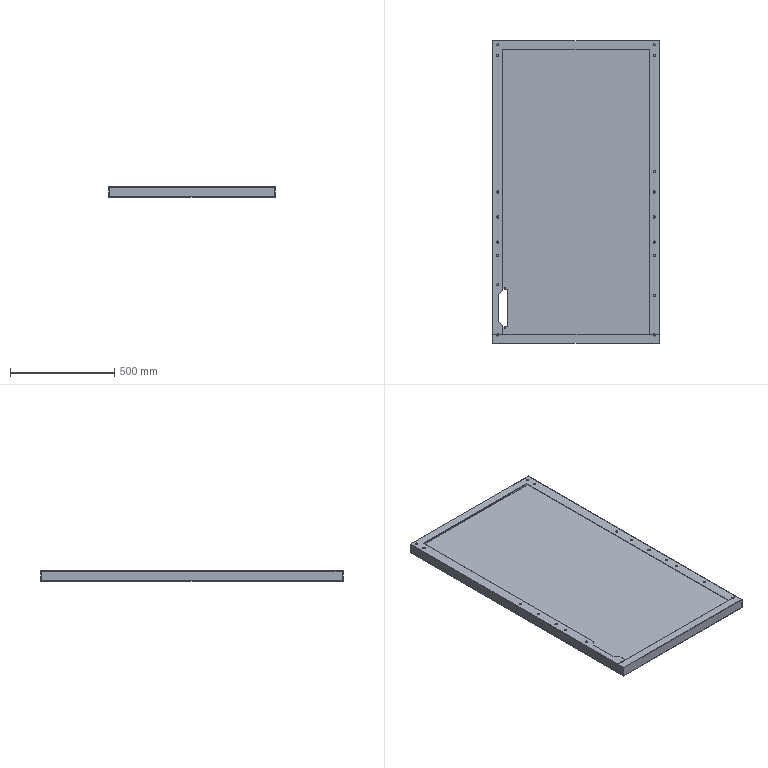Part | SolidWorks | features BaseBody 1 | 1 solid | 69 faces | box 800 x 1450 x 50 mm | volume 3876039 mm3 | cylinder 38 | plane 31 | commonest cylinder face diameters 10.6 x34 4.4 x4